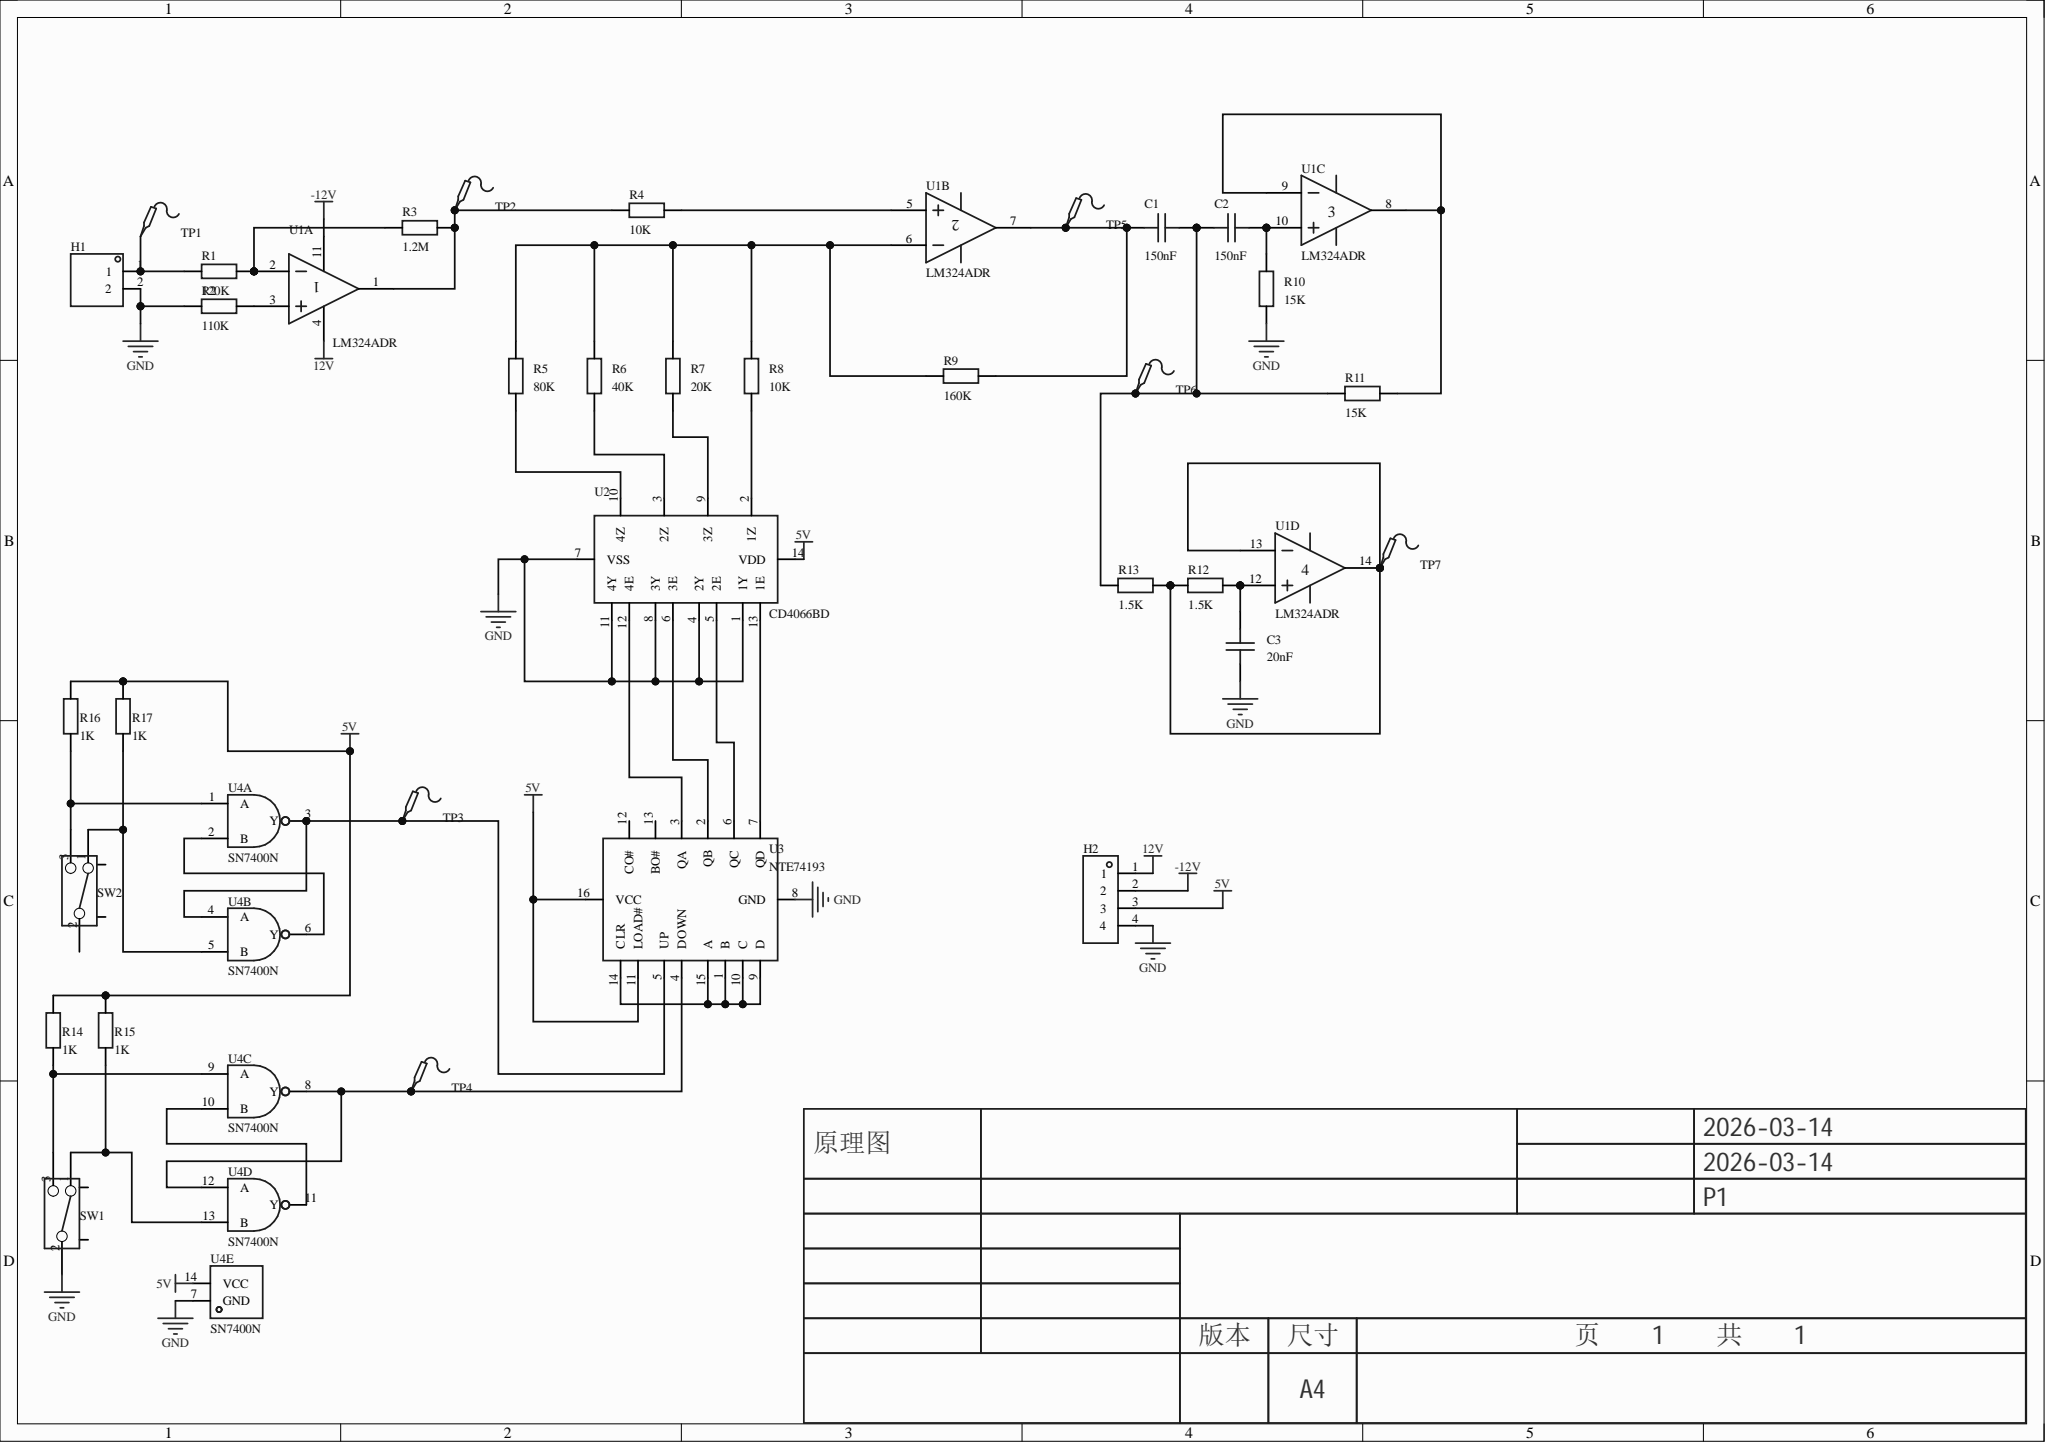Circuit board | Altium Designer | 35 parts | 33 nets
Bill of materials:
Comment,Description,Designator,Footprint,LibRef,Quantity
"150nF","","C1, C2","C0603","CAP_0603","2"
"20nF","","C3","C0603","CAP_0603","1"
"","","H1","HDR-TH_2P-P2.54-V-M-1","HDR-M_2.54_1x2P","1"
"","","H2","HDR-TH_4P-P2.54-V-M","HDR-M_2.54_1x4P","1"
"120K","","R1","R0603","Res_0603","1"
"110K","","R2","R0603","Res_0603","1"
"1.2M","","R3","R0603","Res_0603","1"
"10K","","R4, R8","R0603","Res_0603","2"
"80K","","R5","R0603","Res_0603","1"
"40K","","R6","R0603","Res_0603","1"
"20K","","R7","R0603","Res_0603","1"
"160K","","R9","R0603","Res_0603","1"
"15K","","R10, R11","R0603","Res_0603","2"
"1.5K","","R12, R13","R0603","Res_0603","2"
"1K","","R14, R15, R16, R17","R0603","Res_0603","4"
"","","SW1, SW2","拨动开关_侧","拨动开关_侧","2"
"","Test Point 测试点","TP1, TP2, TP3, TP4, TP5, TP6, TP7","Test-Point-0.5mm","Test-Point","7"
"LM324ADR","放大器数:四路;轨到轨:-;增益带宽积(GBP):-;输入失调电压(Vos):9mV;输入偏置电流(Ib):250nA;","U1","SOP-14_L8.6-W3.9-P1.27-LS6.0-BL","LM324ADR_C2837469","1"
"CD4066BD","","U2","SOP-14_L8.6-W3.9-P1.27-LS6.0-BL","CD4066BD","1"
"NTE74193","工作电压:-;元件数:1;计数速率:32MHz;","U3","PDIP-16_L19.7-W6.6-P2.54-LS7.6-BL","NTE74193","1"
"SN7400N","逻辑类型:与非门;通道数:4;电源电压:4.75V~5.25V;最大传播延迟:22ns@5V,15pF;","U4","PDIP-14_L19.3-W6.4-P2.54-LS7.9-BL-1","SN7400N","1"
Netlist (Protel format):
[
C1
C0603
150nF



]
[
C2
C0603
150nF



]
[
C3
C0603
20nF



]
[
H1
HDR-TH_2P-P2.54-V-M-1




]
[
H2
HDR-TH_4P-P2.54-V-M




]
[
R1
R0603
120K



]
[
R2
R0603
110K



]
[
R3
R0603
1.2M



]
[
R4
R0603
10K



]
[
R5
R0603
80K



]
[
R6
R0603
40K



]
[
R7
R0603
20K



]
[
R8
R0603
10K



]
[
R9
R0603
160K



]
[
R10
R0603
15K



]
[
R11
R0603
15K



]
[
R12
R0603
1.5K



]
[
R13
R0603
1.5K



]
[
R14
R0603
1K



]
[
R15
R0603
1K



]
[
R16
R0603
1K



]
[
R17
R0603
1K



]
[
SW1
拨动开关_侧




]
[
SW2
拨动开关_侧




]
[
TP1
Test-Point-0.5mm




]
[
TP2
Test-Point-0.5mm




]
[
TP3
Test-Point-0.5mm




]
[
TP4
Test-Point-0.5mm




]
[
TP5
Test-Point-0.5mm




]
[
TP6
Test-Point-0.5mm




]
[
TP7
Test-Point-0.5mm




]
[
U1
SOP-14_L8.6-W3.9-P1.27-LS6.0-BL
LM324ADR



]
[
U2
SOP-14_L8.6-W3.9-P1.27-LS6.0-BL
CD4066BD



]
[
U3
PDIP-16_L19.7-W6.6-P2.54-LS7.6-BL
NTE74193



]
[
U4
PDIP-14_L19.3-W6.4-P2.54-LS7.9-BL-1
SN7400N



]
(
NetU4_10
U4-10
U4-11
)
(
NetU4_2
U4-2
U4-6
)
(
NetU3_1
U3-1
U3-9
U3-10
U3-14
U3-15
)
(
NetU2_13
U2-13
U3-7
)
(
NetU2_12
U2-12
U3-3
)
(
NetU2_6
U2-6
U3-2
)
(
NetU2_5
U2-5
U3-6
)
(
NetTP4_1
TP4-1
U3-4
U4-8
U4-12
)
(
NetTP3_1
TP3-1
U3-5
U4-3
U4-4
)
(
NetR17_1
R17-1
SW2-1
U4-5
)
(
NetR16_1
R16-1
SW2-3
U4-1
)
(
NetR15_1
R15-1
SW1-1
U4-13
)
(
NetR14_1
R14-1
SW1-3
U4-9
)
(
NetR12_1
R12-1
R13-2
TP7-1
U1-13
U1-14
)
(
NetR11_1
R11-1
U1-8
U1-9
)
(
NetR8_1
R8-1
U2-2
)
(
NetR7_1
R7-1
U2-9
)
(
NetR6_1
R6-1
U2-3
)
(
NetR5_2
R5-2
R6-2
R7-2
R8-2
R9-2
U1-6
)
(
NetR5_1
R5-1
U2-10
)
(
NetR4_2
R4-2
U1-5
)
(
NetR3_2
R3-2
R4-1
TP2-1
U1-1
)
(
NetR2_2
R2-2
U1-3
)
(
NetR1_2
R1-2
R3-1
U1-2
)
(
NetH1_1
H1-1
R1-1
TP1-1
)
(
NetC3_2
C3-2
R12-2
U1-12
)
(
NetC2_2
C2-2
R10-2
U1-10
)
(
NetC1_2
C1-2
C2-1
R11-2
R13-1
TP6-1
)
(
NetC1_1
C1-1
R9-1
TP5-1
U1-7
)
(
GND
C3-1
H1-2
H2-4
R2-1
R10-1
SW1-2
U2-1
U2-4
U2-7
U2-8
U2-11
U3-8
U4-7
)
(
-12V
H2-2
U1-11
)
(
12V
H2-1
U1-4
)
(
5V
H2-3
R14-2
R15-2
R16-2
R17-2
U2-14
U3-11
U3-16
U4-14
)